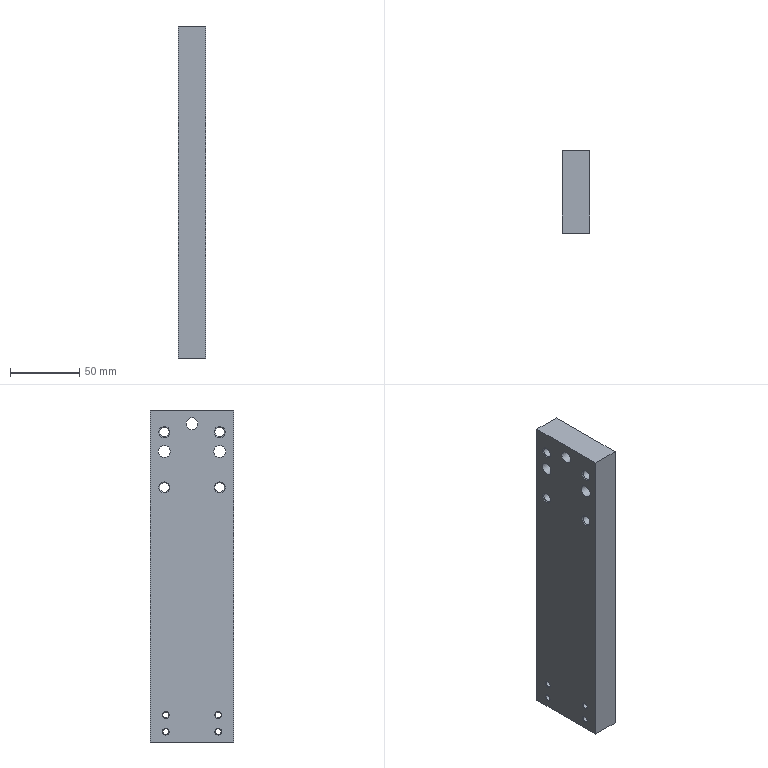Part | STEP file | 冲床-300配套压波_id734_x_t | 1 solid | 31 faces | box 20 x 60 x 240 mm | volume 277564 mm3 | cylinder 14 | plane 9 | cone 8 | commonest cylinder face diameters 4.2 x4 6.8 x4 8.7 x3 14 x3
STEP:
#1=CARTESIAN_POINT('',(1945.,20.,-348.));
#2=VERTEX_POINT('',#1);
#3=CARTESIAN_POINT('',(1945.,20.,-355.));
#4=DIRECTION('',(1.,0.,0.));
#5=DIRECTION('',(0.,0.,1.));
#6=AXIS2_PLACEMENT_3D('',#3,#4,#5);
#7=CIRCLE('',#6,7.);
#8=EDGE_CURVE('',#2,#2,#7,.T.);
#9=ORIENTED_EDGE('',*,*,#8,.T.);
#10=EDGE_LOOP('',(#9));
#11=FACE_BOUND('',#10,.T.);
#12=CARTESIAN_POINT('',(1945.,20.,-350.65));
#13=VERTEX_POINT('',#12);
#14=CARTESIAN_POINT('',(1945.,20.,-355.));
#15=DIRECTION('',(1.,0.,0.));
#16=DIRECTION('',(0.,0.,1.));
#17=AXIS2_PLACEMENT_3D('',#14,#15,#16);
#18=CIRCLE('',#17,4.35);
#19=EDGE_CURVE('',#13,#13,#18,.T.);
#20=ORIENTED_EDGE('',*,*,#19,.F.);
#21=EDGE_LOOP('',(#20));
#22=FACE_BOUND('',#21,.T.);
#23=CARTESIAN_POINT('',(1945.,20.,-355.));
#24=DIRECTION('',(-1.,0.,0.));
#25=DIRECTION('',(0.,0.,1.));
#26=AXIS2_PLACEMENT_3D('',#23,#24,#25);
#27=PLANE('',#26);
#28=ADVANCED_FACE('',(#11,#22),#27,.F.);
#29=CARTESIAN_POINT('',(1955.,20.,-362.));
#30=VERTEX_POINT('',#29);
#31=CARTESIAN_POINT('',(1955.,20.,-355.));
#32=DIRECTION('',(-1.,0.,0.));
#33=DIRECTION('',(0.,0.,-1.));
#34=AXIS2_PLACEMENT_3D('',#31,#32,#33);
#35=CIRCLE('',#34,7.);
#36=EDGE_CURVE('',#30,#30,#35,.T.);
#37=ORIENTED_EDGE('',*,*,#36,.F.);
#38=EDGE_LOOP('',(#37));
#39=FACE_BOUND('',#38,.T.);
#40=ORIENTED_EDGE('',*,*,#8,.F.);
#41=EDGE_LOOP('',(#40));
#42=FACE_BOUND('',#41,.T.);
#43=CARTESIAN_POINT('',(1955.,20.,-355.));
#44=DIRECTION('',(-1.,0.,0.));
#45=DIRECTION('',(0.,0.,1.));
#46=AXIS2_PLACEMENT_3D('',#43,#44,#45);
#47=CYLINDRICAL_SURFACE('',#46,7.);
#48=ADVANCED_FACE('',(#39,#42),#47,.F.);
#49=CARTESIAN_POINT('',(1945.,-20.,-348.));
#50=VERTEX_POINT('',#49);
#51=CARTESIAN_POINT('',(1945.,-20.,-355.));
#52=DIRECTION('',(1.,0.,0.));
#53=DIRECTION('',(0.,0.,1.));
#54=AXIS2_PLACEMENT_3D('',#51,#52,#53);
#55=CIRCLE('',#54,7.);
#56=EDGE_CURVE('',#50,#50,#55,.T.);
#57=ORIENTED_EDGE('',*,*,#56,.T.);
#58=EDGE_LOOP('',(#57));
#59=FACE_BOUND('',#58,.T.);
#60=CARTESIAN_POINT('',(1945.,-20.,-350.65));
#61=VERTEX_POINT('',#60);
#62=CARTESIAN_POINT('',(1945.,-20.,-355.));
#63=DIRECTION('',(1.,0.,0.));
#64=DIRECTION('',(0.,0.,1.));
#65=AXIS2_PLACEMENT_3D('',#62,#63,#64);
#66=CIRCLE('',#65,4.35);
#67=EDGE_CURVE('',#61,#61,#66,.T.);
#68=ORIENTED_EDGE('',*,*,#67,.F.);
#69=EDGE_LOOP('',(#68));
#70=FACE_BOUND('',#69,.T.);
#71=CARTESIAN_POINT('',(1945.,-20.,-355.));
#72=DIRECTION('',(-1.,0.,0.));
#73=DIRECTION('',(0.,0.,1.));
#74=AXIS2_PLACEMENT_3D('',#71,#72,#73);
#75=PLANE('',#74);
#76=ADVANCED_FACE('',(#59,#70),#75,.F.);
#77=CARTESIAN_POINT('',(1955.,-20.,-362.));
#78=VERTEX_POINT('',#77);
#79=CARTESIAN_POINT('',(1955.,-20.,-355.));
#80=DIRECTION('',(-1.,0.,0.));
#81=DIRECTION('',(0.,0.,-1.));
#82=AXIS2_PLACEMENT_3D('',#79,#80,#81);
#83=CIRCLE('',#82,7.);
#84=EDGE_CURVE('',#78,#78,#83,.T.);
#85=ORIENTED_EDGE('',*,*,#84,.F.);
#86=EDGE_LOOP('',(#85));
#87=FACE_BOUND('',#86,.T.);
#88=ORIENTED_EDGE('',*,*,#56,.F.);
#89=EDGE_LOOP('',(#88));
#90=FACE_BOUND('',#89,.T.);
#91=CARTESIAN_POINT('',(1955.,-20.,-355.));
#92=DIRECTION('',(-1.,0.,0.));
#93=DIRECTION('',(0.,0.,1.));
#94=AXIS2_PLACEMENT_3D('',#91,#92,#93);
#95=CYLINDRICAL_SURFACE('',#94,7.);
#96=ADVANCED_FACE('',(#87,#90),#95,.F.);
#97=CARTESIAN_POINT('',(1955.,-30.,-565.));
#98=VERTEX_POINT('',#97);
#99=CARTESIAN_POINT('',(1955.,30.,-565.));
#100=VERTEX_POINT('',#99);
#101=CARTESIAN_POINT('',(1955.,0.,-565.));
#102=DIRECTION('',(0.,1.,0.));
#103=VECTOR('',#102,1.);
#104=LINE('',#101,#103);
#105=EDGE_CURVE('',#98,#100,#104,.T.);
#106=ORIENTED_EDGE('',*,*,#105,.F.);
#107=CARTESIAN_POINT('',(1935.,-30.,-565.));
#108=VERTEX_POINT('',#107);
#109=CARTESIAN_POINT('',(1935.,-30.,-565.));
#110=DIRECTION('',(-1.,0.,0.));
#111=VECTOR('',#110,1.);
#112=LINE('',#109,#111);
#113=EDGE_CURVE('',#98,#108,#112,.T.);
#114=ORIENTED_EDGE('',*,*,#113,.T.);
#115=CARTESIAN_POINT('',(1935.,30.,-565.));
#116=VERTEX_POINT('',#115);
#117=CARTESIAN_POINT('',(1935.,0.,-565.));
#118=DIRECTION('',(0.,1.,0.));
#119=VECTOR('',#118,1.);
#120=LINE('',#117,#119);
#121=EDGE_CURVE('',#108,#116,#120,.T.);
#122=ORIENTED_EDGE('',*,*,#121,.T.);
#123=CARTESIAN_POINT('',(1935.,30.,-565.));
#124=DIRECTION('',(1.,0.,0.));
#125=VECTOR('',#124,1.);
#126=LINE('',#123,#125);
#127=EDGE_CURVE('',#116,#100,#126,.T.);
#128=ORIENTED_EDGE('',*,*,#127,.T.);
#129=EDGE_LOOP('',(#106,#114,#122,#128));
#130=FACE_OUTER_BOUND('',#129,.T.);
#131=CARTESIAN_POINT('',(1935.,-20.,-565.));
#132=DIRECTION('',(0.,0.,-1.));
#133=DIRECTION('',(-1.,0.,0.));
#134=AXIS2_PLACEMENT_3D('',#131,#132,#133);
#135=PLANE('',#134);
#136=ADVANCED_FACE('',(#130),#135,.T.);
#137=CARTESIAN_POINT('',(1935.,-30.,-325.));
#138=VERTEX_POINT('',#137);
#139=CARTESIAN_POINT('',(1935.,-30.,10.));
#140=DIRECTION('',(0.,0.,-1.));
#141=VECTOR('',#140,1.);
#142=LINE('',#139,#141);
#143=EDGE_CURVE('',#138,#108,#142,.T.);
#144=ORIENTED_EDGE('',*,*,#143,.T.);
#145=ORIENTED_EDGE('',*,*,#113,.F.);
#146=CARTESIAN_POINT('',(1955.,-30.,-325.));
#147=VERTEX_POINT('',#146);
#148=CARTESIAN_POINT('',(1955.,-30.,10.));
#149=DIRECTION('',(0.,0.,-1.));
#150=VECTOR('',#149,1.);
#151=LINE('',#148,#150);
#152=EDGE_CURVE('',#147,#98,#151,.T.);
#153=ORIENTED_EDGE('',*,*,#152,.F.);
#154=CARTESIAN_POINT('',(1935.,-30.,-325.));
#155=DIRECTION('',(-1.,0.,0.));
#156=VECTOR('',#155,1.);
#157=LINE('',#154,#156);
#158=EDGE_CURVE('',#147,#138,#157,.T.);
#159=ORIENTED_EDGE('',*,*,#158,.T.);
#160=EDGE_LOOP('',(#144,#145,#153,#159));
#161=FACE_OUTER_BOUND('',#160,.T.);
#162=CARTESIAN_POINT('',(1935.,-30.,-370.));
#163=DIRECTION('',(0.,-1.,0.));
#164=DIRECTION('',(0.,0.,-1.));
#165=AXIS2_PLACEMENT_3D('',#162,#163,#164);
#166=PLANE('',#165);
#167=ADVANCED_FACE('',(#161),#166,.T.);
#168=CARTESIAN_POINT('',(1935.,19.,-548.));
#169=VERTEX_POINT('',#168);
#170=CARTESIAN_POINT('',(1935.,19.,-545.5));
#171=DIRECTION('',(1.,0.,0.));
#172=DIRECTION('',(0.,0.,-1.));
#173=AXIS2_PLACEMENT_3D('',#170,#171,#172);
#174=CIRCLE('',#173,2.5);
#175=EDGE_CURVE('',#169,#169,#174,.T.);
#176=ORIENTED_EDGE('',*,*,#175,.T.);
#177=EDGE_LOOP('',(#176));
#178=FACE_BOUND('',#177,.T.);
#179=CARTESIAN_POINT('',(1935.,19.,-560.));
#180=VERTEX_POINT('',#179);
#181=CARTESIAN_POINT('',(1935.,19.,-557.5));
#182=DIRECTION('',(1.,0.,0.));
#183=DIRECTION('',(0.,0.,-1.));
#184=AXIS2_PLACEMENT_3D('',#181,#182,#183);
#185=CIRCLE('',#184,2.5);
#186=EDGE_CURVE('',#180,#180,#185,.T.);
#187=ORIENTED_EDGE('',*,*,#186,.T.);
#188=EDGE_LOOP('',(#187));
#189=FACE_BOUND('',#188,.T.);
#190=CARTESIAN_POINT('',(1935.,-19.,-560.));
#191=VERTEX_POINT('',#190);
#192=CARTESIAN_POINT('',(1935.,-19.,-557.5));
#193=DIRECTION('',(1.,0.,0.));
#194=DIRECTION('',(0.,0.,-1.));
#195=AXIS2_PLACEMENT_3D('',#192,#193,#194);
#196=CIRCLE('',#195,2.5);
#197=EDGE_CURVE('',#191,#191,#196,.T.);
#198=ORIENTED_EDGE('',*,*,#197,.T.);
#199=EDGE_LOOP('',(#198));
#200=FACE_BOUND('',#199,.T.);
#201=CARTESIAN_POINT('',(1935.,-19.,-548.));
#202=VERTEX_POINT('',#201);
#203=CARTESIAN_POINT('',(1935.,-19.,-545.5));
#204=DIRECTION('',(1.,0.,0.));
#205=DIRECTION('',(0.,0.,-1.));
#206=AXIS2_PLACEMENT_3D('',#203,#204,#205);
#207=CIRCLE('',#206,2.5);
#208=EDGE_CURVE('',#202,#202,#207,.T.);
#209=ORIENTED_EDGE('',*,*,#208,.T.);
#210=EDGE_LOOP('',(#209));
#211=FACE_BOUND('',#210,.T.);
#212=CARTESIAN_POINT('',(1935.,20.,-359.35));
#213=VERTEX_POINT('',#212);
#214=CARTESIAN_POINT('',(1935.,20.,-355.));
#215=DIRECTION('',(1.,0.,0.));
#216=DIRECTION('',(0.,0.,-1.));
#217=AXIS2_PLACEMENT_3D('',#214,#215,#216);
#218=CIRCLE('',#217,4.35);
#219=EDGE_CURVE('',#213,#213,#218,.T.);
#220=ORIENTED_EDGE('',*,*,#219,.T.);
#221=EDGE_LOOP('',(#220));
#222=FACE_BOUND('',#221,.T.);
#223=CARTESIAN_POINT('',(1935.,-20.,-359.35));
#224=VERTEX_POINT('',#223);
#225=CARTESIAN_POINT('',(1935.,-20.,-355.));
#226=DIRECTION('',(1.,0.,0.));
#227=DIRECTION('',(0.,0.,-1.));
#228=AXIS2_PLACEMENT_3D('',#225,#226,#227);
#229=CIRCLE('',#228,4.35);
#230=EDGE_CURVE('',#224,#224,#229,.T.);
#231=ORIENTED_EDGE('',*,*,#230,.T.);
#232=EDGE_LOOP('',(#231));
#233=FACE_BOUND('',#232,.T.);
#234=CARTESIAN_POINT('',(1935.,0.,-339.35));
#235=VERTEX_POINT('',#234);
#236=CARTESIAN_POINT('',(1935.,0.,-335.));
#237=DIRECTION('',(1.,0.,0.));
#238=DIRECTION('',(0.,0.,-1.));
#239=AXIS2_PLACEMENT_3D('',#236,#237,#238);
#240=CIRCLE('',#239,4.35);
#241=EDGE_CURVE('',#235,#235,#240,.T.);
#242=ORIENTED_EDGE('',*,*,#241,.T.);
#243=EDGE_LOOP('',(#242));
#244=FACE_BOUND('',#243,.T.);
#245=CARTESIAN_POINT('',(1935.,20.,-385.));
#246=VERTEX_POINT('',#245);
#247=CARTESIAN_POINT('',(1935.,20.,-381.));
#248=DIRECTION('',(1.,0.,0.));
#249=DIRECTION('',(0.,0.,-1.));
#250=AXIS2_PLACEMENT_3D('',#247,#248,#249);
#251=CIRCLE('',#250,4.);
#252=EDGE_CURVE('',#246,#246,#251,.T.);
#253=ORIENTED_EDGE('',*,*,#252,.T.);
#254=EDGE_LOOP('',(#253));
#255=FACE_BOUND('',#254,.T.);
#256=CARTESIAN_POINT('',(1935.,-20.,-385.));
#257=VERTEX_POINT('',#256);
#258=CARTESIAN_POINT('',(1935.,-20.,-381.));
#259=DIRECTION('',(1.,0.,0.));
#260=DIRECTION('',(0.,0.,-1.));
#261=AXIS2_PLACEMENT_3D('',#258,#259,#260);
#262=CIRCLE('',#261,4.);
#263=EDGE_CURVE('',#257,#257,#262,.T.);
#264=ORIENTED_EDGE('',*,*,#263,.T.);
#265=EDGE_LOOP('',(#264));
#266=FACE_BOUND('',#265,.T.);
#267=CARTESIAN_POINT('',(1935.,20.,-345.));
#268=VERTEX_POINT('',#267);
#269=CARTESIAN_POINT('',(1935.,20.,-341.));
#270=DIRECTION('',(1.,0.,0.));
#271=DIRECTION('',(0.,0.,-1.));
#272=AXIS2_PLACEMENT_3D('',#269,#270,#271);
#273=CIRCLE('',#272,4.);
#274=EDGE_CURVE('',#268,#268,#273,.T.);
#275=ORIENTED_EDGE('',*,*,#274,.T.);
#276=EDGE_LOOP('',(#275));
#277=FACE_BOUND('',#276,.T.);
#278=CARTESIAN_POINT('',(1935.,-20.,-345.));
#279=VERTEX_POINT('',#278);
#280=CARTESIAN_POINT('',(1935.,-20.,-341.));
#281=DIRECTION('',(1.,0.,0.));
#282=DIRECTION('',(0.,0.,-1.));
#283=AXIS2_PLACEMENT_3D('',#280,#281,#282);
#284=CIRCLE('',#283,4.);
#285=EDGE_CURVE('',#279,#279,#284,.T.);
#286=ORIENTED_EDGE('',*,*,#285,.T.);
#287=EDGE_LOOP('',(#286));
#288=FACE_BOUND('',#287,.T.);
#289=ORIENTED_EDGE('',*,*,#143,.F.);
#290=CARTESIAN_POINT('',(1935.,30.,-325.));
#291=VERTEX_POINT('',#290);
#292=CARTESIAN_POINT('',(1935.,0.,-325.));
#293=DIRECTION('',(0.,-1.,0.));
#294=VECTOR('',#293,1.);
#295=LINE('',#292,#294);
#296=EDGE_CURVE('',#291,#138,#295,.T.);
#297=ORIENTED_EDGE('',*,*,#296,.F.);
#298=CARTESIAN_POINT('',(1935.,30.,10.));
#299=DIRECTION('',(0.,0.,1.));
#300=VECTOR('',#299,1.);
#301=LINE('',#298,#300);
#302=EDGE_CURVE('',#116,#291,#301,.T.);
#303=ORIENTED_EDGE('',*,*,#302,.F.);
#304=ORIENTED_EDGE('',*,*,#121,.F.);
#305=EDGE_LOOP('',(#289,#297,#303,#304));
#306=FACE_BOUND('',#305,.T.);
#307=CARTESIAN_POINT('',(1935.,0.,10.));
#308=DIRECTION('',(1.,0.,0.));
#309=DIRECTION('',(0.,0.,-1.));
#310=AXIS2_PLACEMENT_3D('',#307,#308,#309);
#311=PLANE('',#310);
#312=ADVANCED_FACE('',(#178,#189,#200,#211,#222,#233,#244,#255,#266,#277,#288,#306),#311,.F.);
#313=CARTESIAN_POINT('',(1955.,30.,-325.));
#314=VERTEX_POINT('',#313);
#315=CARTESIAN_POINT('',(1955.,30.,10.));
#316=DIRECTION('',(0.,0.,1.));
#317=VECTOR('',#316,1.);
#318=LINE('',#315,#317);
#319=EDGE_CURVE('',#100,#314,#318,.T.);
#320=ORIENTED_EDGE('',*,*,#319,.F.);
#321=ORIENTED_EDGE('',*,*,#127,.F.);
#322=ORIENTED_EDGE('',*,*,#302,.T.);
#323=CARTESIAN_POINT('',(1935.,30.,-325.));
#324=DIRECTION('',(1.,0.,0.));
#325=VECTOR('',#324,1.);
#326=LINE('',#323,#325);
#327=EDGE_CURVE('',#291,#314,#326,.T.);
#328=ORIENTED_EDGE('',*,*,#327,.T.);
#329=EDGE_LOOP('',(#320,#321,#322,#328));
#330=FACE_OUTER_BOUND('',#329,.T.);
#331=CARTESIAN_POINT('',(1935.,30.,-550.));
#332=DIRECTION('',(0.,1.,0.));
#333=DIRECTION('',(0.,0.,1.));
#334=AXIS2_PLACEMENT_3D('',#331,#332,#333);
#335=PLANE('',#334);
#336=ADVANCED_FACE('',(#330),#335,.T.);
#337=ORIENTED_EDGE('',*,*,#36,.T.);
#338=EDGE_LOOP('',(#337));
#339=FACE_BOUND('',#338,.T.);
#340=ORIENTED_EDGE('',*,*,#84,.T.);
#341=EDGE_LOOP('',(#340));
#342=FACE_BOUND('',#341,.T.);
#343=CARTESIAN_POINT('',(1955.,0.,-342.));
#344=VERTEX_POINT('',#343);
#345=CARTESIAN_POINT('',(1955.,0.,-335.));
#346=DIRECTION('',(-1.,0.,0.));
#347=DIRECTION('',(0.,0.,-1.));
#348=AXIS2_PLACEMENT_3D('',#345,#346,#347);
#349=CIRCLE('',#348,7.);
#350=EDGE_CURVE('',#344,#344,#349,.T.);
#351=ORIENTED_EDGE('',*,*,#350,.T.);
#352=EDGE_LOOP('',(#351));
#353=FACE_BOUND('',#352,.T.);
#354=CARTESIAN_POINT('',(1955.,0.,-325.));
#355=DIRECTION('',(0.,-1.,0.));
#356=VECTOR('',#355,1.);
#357=LINE('',#354,#356);
#358=EDGE_CURVE('',#314,#147,#357,.T.);
#359=ORIENTED_EDGE('',*,*,#358,.T.);
#360=ORIENTED_EDGE('',*,*,#152,.T.);
#361=ORIENTED_EDGE('',*,*,#105,.T.);
#362=ORIENTED_EDGE('',*,*,#319,.T.);
#363=EDGE_LOOP('',(#359,#360,#361,#362));
#364=FACE_BOUND('',#363,.T.);
#365=CARTESIAN_POINT('',(1955.,19.,-547.6));
#366=VERTEX_POINT('',#365);
#367=CARTESIAN_POINT('',(1955.,19.,-545.5));
#368=DIRECTION('',(1.,0.,0.));
#369=DIRECTION('',(0.,0.,-1.));
#370=AXIS2_PLACEMENT_3D('',#367,#368,#369);
#371=CIRCLE('',#370,2.1);
#372=EDGE_CURVE('',#366,#366,#371,.T.);
#373=ORIENTED_EDGE('',*,*,#372,.F.);
#374=EDGE_LOOP('',(#373));
#375=FACE_BOUND('',#374,.T.);
#376=CARTESIAN_POINT('',(1955.,19.,-559.6));
#377=VERTEX_POINT('',#376);
#378=CARTESIAN_POINT('',(1955.,19.,-557.5));
#379=DIRECTION('',(1.,0.,0.));
#380=DIRECTION('',(0.,0.,-1.));
#381=AXIS2_PLACEMENT_3D('',#378,#379,#380);
#382=CIRCLE('',#381,2.1);
#383=EDGE_CURVE('',#377,#377,#382,.T.);
#384=ORIENTED_EDGE('',*,*,#383,.F.);
#385=EDGE_LOOP('',(#384));
#386=FACE_BOUND('',#385,.T.);
#387=CARTESIAN_POINT('',(1955.,-19.,-559.6));
#388=VERTEX_POINT('',#387);
#389=CARTESIAN_POINT('',(1955.,-19.,-557.5));
#390=DIRECTION('',(1.,0.,0.));
#391=DIRECTION('',(0.,0.,-1.));
#392=AXIS2_PLACEMENT_3D('',#389,#390,#391);
#393=CIRCLE('',#392,2.1);
#394=EDGE_CURVE('',#388,#388,#393,.T.);
#395=ORIENTED_EDGE('',*,*,#394,.F.);
#396=EDGE_LOOP('',(#395));
#397=FACE_BOUND('',#396,.T.);
#398=CARTESIAN_POINT('',(1955.,-19.,-547.6));
#399=VERTEX_POINT('',#398);
#400=CARTESIAN_POINT('',(1955.,-19.,-545.5));
#401=DIRECTION('',(1.,0.,0.));
#402=DIRECTION('',(0.,0.,-1.));
#403=AXIS2_PLACEMENT_3D('',#400,#401,#402);
#404=CIRCLE('',#403,2.1);
#405=EDGE_CURVE('',#399,#399,#404,.T.);
#406=ORIENTED_EDGE('',*,*,#405,.F.);
#407=EDGE_LOOP('',(#406));
#408=FACE_BOUND('',#407,.T.);
#409=CARTESIAN_POINT('',(1955.,20.,-344.4));
#410=VERTEX_POINT('',#409);
#411=CARTESIAN_POINT('',(1955.,20.,-341.));
#412=DIRECTION('',(1.,0.,0.));
#413=DIRECTION('',(0.,0.,-1.));
#414=AXIS2_PLACEMENT_3D('',#411,#412,#413);
#415=CIRCLE('',#414,3.4);
#416=EDGE_CURVE('',#410,#410,#415,.T.);
#417=ORIENTED_EDGE('',*,*,#416,.F.);
#418=EDGE_LOOP('',(#417));
#419=FACE_BOUND('',#418,.T.);
#420=CARTESIAN_POINT('',(1955.,-20.,-344.4));
#421=VERTEX_POINT('',#420);
#422=CARTESIAN_POINT('',(1955.,-20.,-341.));
#423=DIRECTION('',(1.,0.,0.));
#424=DIRECTION('',(0.,0.,-1.));
#425=AXIS2_PLACEMENT_3D('',#422,#423,#424);
#426=CIRCLE('',#425,3.4);
#427=EDGE_CURVE('',#421,#421,#426,.T.);
#428=ORIENTED_EDGE('',*,*,#427,.F.);
#429=EDGE_LOOP('',(#428));
#430=FACE_BOUND('',#429,.T.);
#431=CARTESIAN_POINT('',(1955.,20.,-384.4));
#432=VERTEX_POINT('',#431);
#433=CARTESIAN_POINT('',(1955.,20.,-381.));
#434=DIRECTION('',(1.,0.,0.));
#435=DIRECTION('',(0.,0.,-1.));
#436=AXIS2_PLACEMENT_3D('',#433,#434,#435);
#437=CIRCLE('',#436,3.4);
#438=EDGE_CURVE('',#432,#432,#437,.T.);
#439=ORIENTED_EDGE('',*,*,#438,.F.);
#440=EDGE_LOOP('',(#439));
#441=FACE_BOUND('',#440,.T.);
#442=CARTESIAN_POINT('',(1955.,-20.,-384.4));
#443=VERTEX_POINT('',#442);
#444=CARTESIAN_POINT('',(1955.,-20.,-381.));
#445=DIRECTION('',(1.,0.,0.));
#446=DIRECTION('',(0.,0.,-1.));
#447=AXIS2_PLACEMENT_3D('',#444,#445,#446);
#448=CIRCLE('',#447,3.4);
#449=EDGE_CURVE('',#443,#443,#448,.T.);
#450=ORIENTED_EDGE('',*,*,#449,.F.);
#451=EDGE_LOOP('',(#450));
#452=FACE_BOUND('',#451,.T.);
#453=CARTESIAN_POINT('',(1955.,0.,10.));
#454=DIRECTION('',(1.,0.,0.));
#455=DIRECTION('',(0.,0.,-1.));
#456=AXIS2_PLACEMENT_3D('',#453,#454,#455);
#457=PLANE('',#456);
#458=ADVANCED_FACE('',(#339,#342,#353,#364,#375,#386,#397,#408,#419,#430,#441,#452),#457,.T.);
#459=ORIENTED_EDGE('',*,*,#358,.F.);
#460=ORIENTED_EDGE('',*,*,#327,.F.);
#461=ORIENTED_EDGE('',*,*,#296,.T.);
#462=ORIENTED_EDGE('',*,*,#158,.F.);
#463=EDGE_LOOP('',(#459,#460,#461,#462));
#464=FACE_OUTER_BOUND('',#463,.T.);
#465=CARTESIAN_POINT('',(1935.,20.,-325.));
#466=DIRECTION('',(0.,0.,1.));
#467=DIRECTION('',(1.,0.,0.));
#468=AXIS2_PLACEMENT_3D('',#465,#466,#467);
#469=PLANE('',#468);
#470=ADVANCED_FACE('',(#464),#469,.T.);
#471=CARTESIAN_POINT('',(1935.6,-20.,-344.4));
#472=VERTEX_POINT('',#471);
#473=CARTESIAN_POINT('',(1935.6,-20.,-341.));
#474=DIRECTION('',(-1.,0.,0.));
#475=DIRECTION('',(0.,0.,-1.));
#476=AXIS2_PLACEMENT_3D('',#473,#474,#475);
#477=CIRCLE('',#476,3.4);
#478=EDGE_CURVE('',#472,#472,#477,.T.);
#479=ORIENTED_EDGE('',*,*,#478,.T.);
#480=EDGE_LOOP('',(#479));
#481=FACE_BOUND('',#480,.T.);
#482=ORIENTED_EDGE('',*,*,#427,.T.);
#483=EDGE_LOOP('',(#482));
#484=FACE_BOUND('',#483,.T.);
#485=CARTESIAN_POINT('',(1955.,-20.,-341.));
#486=DIRECTION('',(-1.,0.,0.));
#487=DIRECTION('',(0.,0.,1.));
#488=AXIS2_PLACEMENT_3D('',#485,#486,#487);
#489=CYLINDRICAL_SURFACE('',#488,3.4);
#490=ADVANCED_FACE('',(#481,#484),#489,.F.);
#491=ORIENTED_EDGE('',*,*,#478,.F.);
#492=EDGE_LOOP('',(#491));
#493=FACE_BOUND('',#492,.T.);
#494=ORIENTED_EDGE('',*,*,#285,.F.);
#495=EDGE_LOOP('',(#494));
#496=FACE_BOUND('',#495,.T.);
#497=CARTESIAN_POINT('',(1935.,-20.,-341.));
#498=DIRECTION('',(-1.,0.,0.));
#499=DIRECTION('',(0.,0.,1.));
#500=AXIS2_PLACEMENT_3D('',#497,#498,#499);
#501=CONICAL_SURFACE('',#500,4.,45.);
#502=ADVANCED_FACE('',(#493,#496),#501,.F.);
#503=CARTESIAN_POINT('',(1935.6,20.,-344.4));
#504=VERTEX_POINT('',#503);
#505=CARTESIAN_POINT('',(1935.6,20.,-341.));
#506=DIRECTION('',(-1.,0.,0.));
#507=DIRECTION('',(0.,0.,-1.));
#508=AXIS2_PLACEMENT_3D('',#505,#506,#507);
#509=CIRCLE('',#508,3.4);
#510=EDGE_CURVE('',#504,#504,#509,.T.);
#511=ORIENTED_EDGE('',*,*,#510,.T.);
#512=EDGE_LOOP('',(#511));
#513=FACE_BOUND('',#512,.T.);
#514=ORIENTED_EDGE('',*,*,#416,.T.);
#515=EDGE_LOOP('',(#514));
#516=FACE_BOUND('',#515,.T.);
#517=CARTESIAN_POINT('',(1955.,20.,-341.));
#518=DIRECTION('',(-1.,0.,0.));
#519=DIRECTION('',(0.,0.,1.));
#520=AXIS2_PLACEMENT_3D('',#517,#518,#519);
#521=CYLINDRICAL_SURFACE('',#520,3.4);
#522=ADVANCED_FACE('',(#513,#516),#521,.F.);
#523=ORIENTED_EDGE('',*,*,#510,.F.);
#524=EDGE_LOOP('',(#523));
#525=FACE_BOUND('',#524,.T.);
#526=ORIENTED_EDGE('',*,*,#274,.F.);
#527=EDGE_LOOP('',(#526));
#528=FACE_BOUND('',#527,.T.);
#529=CARTESIAN_POINT('',(1935.,20.,-341.));
#530=DIRECTION('',(-1.,0.,0.));
#531=DIRECTION('',(0.,0.,1.));
#532=AXIS2_PLACEMENT_3D('',#529,#530,#531);
#533=CONICAL_SURFACE('',#532,4.,45.);
#534=ADVANCED_FACE('',(#525,#528),#533,.F.);
#535=CARTESIAN_POINT('',(1935.6,-20.,-384.4));
#536=VERTEX_POINT('',#535);
#537=CARTESIAN_POINT('',(1935.6,-20.,-381.));
#538=DIRECTION('',(-1.,0.,0.));
#539=DIRECTION('',(0.,0.,-1.));
#540=AXIS2_PLACEMENT_3D('',#537,#538,#539);
#541=CIRCLE('',#540,3.4);
#542=EDGE_CURVE('',#536,#536,#541,.T.);
#543=ORIENTED_EDGE('',*,*,#542,.T.);
#544=EDGE_LOOP('',(#543));
#545=FACE_BOUND('',#544,.T.);
#546=ORIENTED_EDGE('',*,*,#449,.T.);
#547=EDGE_LOOP('',(#546));
#548=FACE_BOUND('',#547,.T.);
#549=CARTESIAN_POINT('',(1955.,-20.,-381.));
#550=DIRECTION('',(-1.,0.,0.));
#551=DIRECTION('',(0.,0.,1.));
#552=AXIS2_PLACEMENT_3D('',#549,#550,#551);
#553=CYLINDRICAL_SURFACE('',#552,3.4);
#554=ADVANCED_FACE('',(#545,#548),#553,.F.);
#555=ORIENTED_EDGE('',*,*,#542,.F.);
#556=EDGE_LOOP('',(#555));
#557=FACE_BOUND('',#556,.T.);
#558=ORIENTED_EDGE('',*,*,#263,.F.);
#559=EDGE_LOOP('',(#558));
#560=FACE_BOUND('',#559,.T.);
#561=CARTESIAN_POINT('',(1935.,-20.,-381.));
#562=DIRECTION('',(-1.,0.,0.));
#563=DIRECTION('',(0.,0.,1.));
#564=AXIS2_PLACEMENT_3D('',#561,#562,#563);
#565=CONICAL_SURFACE('',#564,4.,45.);
#566=ADVANCED_FACE('',(#557,#560),#565,.F.);
#567=CARTESIAN_POINT('',(1935.6,20.,-384.4));
#568=VERTEX_POINT('',#567);
#569=CARTESIAN_POINT('',(1935.6,20.,-381.));
#570=DIRECTION('',(-1.,0.,0.));
#571=DIRECTION('',(0.,0.,-1.));
#572=AXIS2_PLACEMENT_3D('',#569,#570,#571);
#573=CIRCLE('',#572,3.4);
#574=EDGE_CURVE('',#568,#568,#573,.T.);
#575=ORIENTED_EDGE('',*,*,#574,.T.);
#576=EDGE_LOOP('',(#575));
#577=FACE_BOUND('',#576,.T.);
#578=ORIENTED_EDGE('',*,*,#438,.T.);
#579=EDGE_LOOP('',(#578));
#580=FACE_BOUND('',#579,.T.);
#581=CARTESIAN_POINT('',(1955.,20.,-381.));
#582=DIRECTION('',(-1.,0.,0.));
#583=DIRECTION('',(0.,0.,1.));
#584=AXIS2_PLACEMENT_3D('',#581,#582,#583);
#585=CYLINDRICAL_SURFACE('',#584,3.4);
#586=ADVANCED_FACE('',(#577,#580),#585,.F.);
#587=ORIENTED_EDGE('',*,*,#574,.F.);
#588=EDGE_LOOP('',(#587));
#589=FACE_BOUND('',#588,.T.);
#590=ORIENTED_EDGE('',*,*,#252,.F.);
#591=EDGE_LOOP('',(#590));
#592=FACE_BOUND('',#591,.T.);
#593=CARTESIAN_POINT('',(1935.,20.,-381.));
#594=DIRECTION('',(-1.,0.,0.));
#595=DIRECTION('',(0.,0.,1.));
#596=AXIS2_PLACEMENT_3D('',#593,#594,#595);
#597=CONICAL_SURFACE('',#596,4.,45.);
#598=ADVANCED_FACE('',(#589,#592),#597,.F.);
#599=CARTESIAN_POINT('',(1945.,0.,-330.65));
#600=VERTEX_POINT('',#599);
#601=CARTESIAN_POINT('',(1945.,0.,-335.));
#602=DIRECTION('',(1.,0.,0.));
#603=DIRECTION('',(0.,0.,1.));
#604=AXIS2_PLACEMENT_3D('',#601,#602,#603);
#605=CIRCLE('',#604,4.35);
#606=EDGE_CURVE('',#600,#600,#605,.T.);
#607=ORIENTED_EDGE('',*,*,#606,.T.);
#608=EDGE_LOOP('',(#607));
#609=FACE_BOUND('',#608,.T.);
#610=ORIENTED_EDGE('',*,*,#241,.F.);
#611=EDGE_LOOP('',(#610));
#612=FACE_BOUND('',#611,.T.);
#613=CARTESIAN_POINT('',(1864.167,0.,-335.));
#614=DIRECTION('',(-1.,0.,0.));
#615=DIRECTION('',(0.,0.,1.));
#616=AXIS2_PLACEMENT_3D('',#613,#614,#615);
#617=CYLINDRICAL_SURFACE('',#616,4.35);
#618=ADVANCED_FACE('',(#609,#612),#617,.F.);
#619=ORIENTED_EDGE('',*,*,#606,.F.);
#620=EDGE_LOOP('',(#619));
#621=FACE_BOUND('',#620,.T.);
#622=CARTESIAN_POINT('',(1945.,0.,-328.));
#623=VERTEX_POINT('',#622);
#624=CARTESIAN_POINT('',(1945.,0.,-335.));
#625=DIRECTION('',(1.,0.,0.));
#626=DIRECTION('',(0.,0.,1.));
#627=AXIS2_PLACEMENT_3D('',#624,#625,#626);
#628=CIRCLE('',#627,7.);
#629=EDGE_CURVE('',#623,#623,#628,.T.);
#630=ORIENTED_EDGE('',*,*,#629,.T.);
#631=EDGE_LOOP('',(#630));
#632=FACE_BOUND('',#631,.T.);
#633=CARTESIAN_POINT('',(1945.,0.,-335.));
#634=DIRECTION('',(-1.,0.,0.));
#635=DIRECTION('',(0.,0.,1.));
#636=AXIS2_PLACEMENT_3D('',#633,#634,#635);
#637=PLANE('',#636);
#638=ADVANCED_FACE('',(#621,#632),#637,.F.);
#639=ORIENTED_EDGE('',*,*,#629,.F.);
#640=EDGE_LOOP('',(#639));
#641=FACE_BOUND('',#640,.T.);
#642=ORIENTED_EDGE('',*,*,#350,.F.);
#643=EDGE_LOOP('',(#642));
#644=FACE_BOUND('',#643,.T.);
#645=CARTESIAN_POINT('',(1955.,0.,-335.));
#646=DIRECTION('',(-1.,0.,0.));
#647=DIRECTION('',(0.,0.,1.));
#648=AXIS2_PLACEMENT_3D('',#645,#646,#647);
#649=CYLINDRICAL_SURFACE('',#648,7.);
#650=ADVANCED_FACE('',(#641,#644),#649,.F.);
#651=ORIENTED_EDGE('',*,*,#67,.T.);
#652=EDGE_LOOP('',(#651));
#653=FACE_BOUND('',#652,.T.);
#654=ORIENTED_EDGE('',*,*,#230,.F.);
#655=EDGE_LOOP('',(#654));
#656=FACE_BOUND('',#655,.T.);
#657=CARTESIAN_POINT('',(1844.332,-20.,-355.));
#658=DIRECTION('',(-1.,0.,0.));
#659=DIRECTION('',(0.,0.,1.));
#660=AXIS2_PLACEMENT_3D('',#657,#658,#659);
#661=CYLINDRICAL_SURFACE('',#660,4.35);
#662=ADVANCED_FACE('',(#653,#656),#661,.F.);
#663=ORIENTED_EDGE('',*,*,#19,.T.);
#664=EDGE_LOOP('',(#663));
#665=FACE_BOUND('',#664,.T.);
#666=ORIENTED_EDGE('',*,*,#219,.F.);
#667=EDGE_LOOP('',(#666));
#668=FACE_BOUND('',#667,.T.);
#669=CARTESIAN_POINT('',(1844.332,20.,-355.));
#670=DIRECTION('',(-1.,0.,0.));
#671=DIRECTION('',(0.,0.,1.));
#672=AXIS2_PLACEMENT_3D('',#669,#670,#671);
#673=CYLINDRICAL_SURFACE('',#672,4.35);
#674=ADVANCED_FACE('',(#665,#668),#673,.F.);
#675=CARTESIAN_POINT('',(1935.4,-19.,-547.6));
#676=VERTEX_POINT('',#675);
#677=CARTESIAN_POINT('',(1935.4,-19.,-545.5));
#678=DIRECTION('',(-1.,0.,0.));
#679=DIRECTION('',(0.,0.,-1.));
#680=AXIS2_PLACEMENT_3D('',#677,#678,#679);
#681=CIRCLE('',#680,2.1);
#682=EDGE_CURVE('',#676,#676,#681,.T.);
#683=ORIENTED_EDGE('',*,*,#682,.T.);
#684=EDGE_LOOP('',(#683));
#685=FACE_BOUND('',#684,.T.);
#686=ORIENTED_EDGE('',*,*,#405,.T.);
#687=EDGE_LOOP('',(#686));
#688=FACE_BOUND('',#687,.T.);
#689=CARTESIAN_POINT('',(1955.,-19.,-545.5));
#690=DIRECTION('',(-1.,0.,0.));
#691=DIRECTION('',(0.,0.,1.));
#692=AXIS2_PLACEMENT_3D('',#689,#690,#691);
#693=CYLINDRICAL_SURFACE('',#692,2.1);
#694=ADVANCED_FACE('',(#685,#688),#693,.F.);
#695=ORIENTED_EDGE('',*,*,#682,.F.);
#696=EDGE_LOOP('',(#695));
#697=FACE_BOUND('',#696,.T.);
#698=ORIENTED_EDGE('',*,*,#208,.F.);
#699=EDGE_LOOP('',(#698));
#700=FACE_BOUND('',#699,.T.);
#701=CARTESIAN_POINT('',(1935.,-19.,-545.5));
#702=DIRECTION('',(-1.,0.,0.));
#703=DIRECTION('',(0.,0.,1.));
#704=AXIS2_PLACEMENT_3D('',#701,#702,#703);
#705=CONICAL_SURFACE('',#704,2.5,45.);
#706=ADVANCED_FACE('',(#697,#700),#705,.F.);
#707=CARTESIAN_POINT('',(1935.4,-19.,-559.6));
#708=VERTEX_POINT('',#707);
#709=CARTESIAN_POINT('',(1935.4,-19.,-557.5));
#710=DIRECTION('',(-1.,0.,0.));
#711=DIRECTION('',(0.,0.,-1.));
#712=AXIS2_PLACEMENT_3D('',#709,#710,#711);
#713=CIRCLE('',#712,2.1);
#714=EDGE_CURVE('',#708,#708,#713,.T.);
#715=ORIENTED_EDGE('',*,*,#714,.T.);
#716=EDGE_LOOP('',(#715));
#717=FACE_BOUND('',#716,.T.);
#718=ORIENTED_EDGE('',*,*,#394,.T.);
#719=EDGE_LOOP('',(#718));
#720=FACE_BOUND('',#719,.T.);
#721=CARTESIAN_POINT('',(1955.,-19.,-557.5));
#722=DIRECTION('',(-1.,0.,0.));
#723=DIRECTION('',(0.,0.,1.));
#724=AXIS2_PLACEMENT_3D('',#721,#722,#723);
#725=CYLINDRICAL_SURFACE('',#724,2.1);
#726=ADVANCED_FACE('',(#717,#720),#725,.F.);
#727=ORIENTED_EDGE('',*,*,#714,.F.);
#728=EDGE_LOOP('',(#727));
#729=FACE_BOUND('',#728,.T.);
#730=ORIENTED_EDGE('',*,*,#197,.F.);
#731=EDGE_LOOP('',(#730));
#732=FACE_BOUND('',#731,.T.);
#733=CARTESIAN_POINT('',(1935.,-19.,-557.5));
#734=DIRECTION('',(-1.,0.,0.));
#735=DIRECTION('',(0.,0.,1.));
#736=AXIS2_PLACEMENT_3D('',#733,#734,#735);
#737=CONICAL_SURFACE('',#736,2.5,45.);
#738=ADVANCED_FACE('',(#729,#732),#737,.F.);
#739=CARTESIAN_POINT('',(1935.4,19.,-559.6));
#740=VERTEX_POINT('',#739);
#741=CARTESIAN_POINT('',(1935.4,19.,-557.5));
#742=DIRECTION('',(-1.,0.,0.));
#743=DIRECTION('',(0.,0.,-1.));
#744=AXIS2_PLACEMENT_3D('',#741,#742,#743);
#745=CIRCLE('',#744,2.1);
#746=EDGE_CURVE('',#740,#740,#745,.T.);
#747=ORIENTED_EDGE('',*,*,#746,.T.);
#748=EDGE_LOOP('',(#747));
#749=FACE_BOUND('',#748,.T.);
#750=ORIENTED_EDGE('',*,*,#383,.T.);
#751=EDGE_LOOP('',(#750));
#752=FACE_BOUND('',#751,.T.);
#753=CARTESIAN_POINT('',(1955.,19.,-557.5));
#754=DIRECTION('',(-1.,0.,0.));
#755=DIRECTION('',(0.,0.,1.));
#756=AXIS2_PLACEMENT_3D('',#753,#754,#755);
#757=CYLINDRICAL_SURFACE('',#756,2.1);
#758=ADVANCED_FACE('',(#749,#752),#757,.F.);
#759=ORIENTED_EDGE('',*,*,#746,.F.);
#760=EDGE_LOOP('',(#759));
#761=FACE_BOUND('',#760,.T.);
#762=ORIENTED_EDGE('',*,*,#186,.F.);
#763=EDGE_LOOP('',(#762));
#764=FACE_BOUND('',#763,.T.);
#765=CARTESIAN_POINT('',(1935.,19.,-557.5));
#766=DIRECTION('',(-1.,0.,0.));
#767=DIRECTION('',(0.,0.,1.));
#768=AXIS2_PLACEMENT_3D('',#765,#766,#767);
#769=CONICAL_SURFACE('',#768,2.5,45.);
#770=ADVANCED_FACE('',(#761,#764),#769,.F.);
#771=CARTESIAN_POINT('',(1935.4,19.,-547.6));
#772=VERTEX_POINT('',#771);
#773=CARTESIAN_POINT('',(1935.4,19.,-545.5));
#774=DIRECTION('',(-1.,0.,0.));
#775=DIRECTION('',(0.,0.,-1.));
#776=AXIS2_PLACEMENT_3D('',#773,#774,#775);
#777=CIRCLE('',#776,2.1);
#778=EDGE_CURVE('',#772,#772,#777,.T.);
#779=ORIENTED_EDGE('',*,*,#778,.T.);
#780=EDGE_LOOP('',(#779));
#781=FACE_BOUND('',#780,.T.);
#782=ORIENTED_EDGE('',*,*,#372,.T.);
#783=EDGE_LOOP('',(#782));
#784=FACE_BOUND('',#783,.T.);
#785=CARTESIAN_POINT('',(1955.,19.,-545.5));
#786=DIRECTION('',(-1.,0.,0.));
#787=DIRECTION('',(0.,0.,1.));
#788=AXIS2_PLACEMENT_3D('',#785,#786,#787);
#789=CYLINDRICAL_SURFACE('',#788,2.1);
#790=ADVANCED_FACE('',(#781,#784),#789,.F.);
#791=ORIENTED_EDGE('',*,*,#778,.F.);
#792=EDGE_LOOP('',(#791));
#793=FACE_BOUND('',#792,.T.);
#794=ORIENTED_EDGE('',*,*,#175,.F.);
#795=EDGE_LOOP('',(#794));
#796=FACE_BOUND('',#795,.T.);
#797=CARTESIAN_POINT('',(1935.,19.,-545.5));
#798=DIRECTION('',(-1.,0.,0.));
#799=DIRECTION('',(0.,0.,1.));
#800=AXIS2_PLACEMENT_3D('',#797,#798,#799);
#801=CONICAL_SURFACE('',#800,2.5,45.);
#802=ADVANCED_FACE('',(#793,#796),#801,.F.);
#803=CLOSED_SHELL('',(#28,#48,#76,#96,#136,#167,#312,#336,#458,#470,#490,#502,#522,#534,#554,#566,#586,#598,#618,#638,#650,#662,#674,#694,#706,#726,#738,#758,#770,#790,#802));
#804=MANIFOLD_SOLID_BREP('',#803);
#805=(LENGTH_UNIT()NAMED_UNIT(*)SI_UNIT(.MILLI.,.METRE.));
#806=UNCERTAINTY_MEASURE_WITH_UNIT(LENGTH_MEASURE(0.00002),#805,'','');
#807=(NAMED_UNIT(*)PLANE_ANGLE_UNIT()SI_UNIT($,.RADIAN.));
#808=PLANE_ANGLE_MEASURE_WITH_UNIT(PLANE_ANGLE_MEASURE(0.01745),#807);
#809=DIMENSIONAL_EXPONENTS(0.,0.,0.,0.,0.,0.,0.);
#810=(CONVERSION_BASED_UNIT('DEGREE',#808)NAMED_UNIT(#809)PLANE_ANGLE_UNIT());
#811=(NAMED_UNIT(*)SI_UNIT($,.STERADIAN.)SOLID_ANGLE_UNIT());
#812=(GEOMETRIC_REPRESENTATION_CONTEXT(3)GLOBAL_UNCERTAINTY_ASSIGNED_CONTEXT((#806))GLOBAL_UNIT_ASSIGNED_CONTEXT((#805,#810,#811))REPRESENTATION_CONTEXT('',''));
#813=ADVANCED_BREP_SHAPE_REPRESENTATION('',(#804),#812);